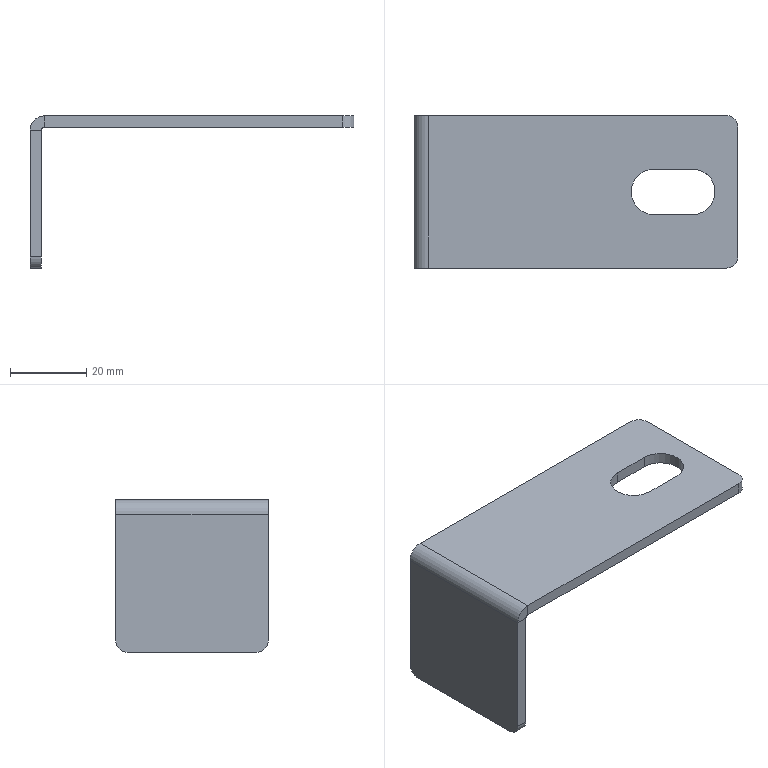Part | STEP file | 粉仓护栏FixedPlate 1 | 1 solid | 23 faces | box 85 x 40 x 40 mm | volume 13802 mm3 | plane 14 | cylinder 9 | commonest cylinder face diameters 6 x4 12 x3 1.473 x1 7.473 x1